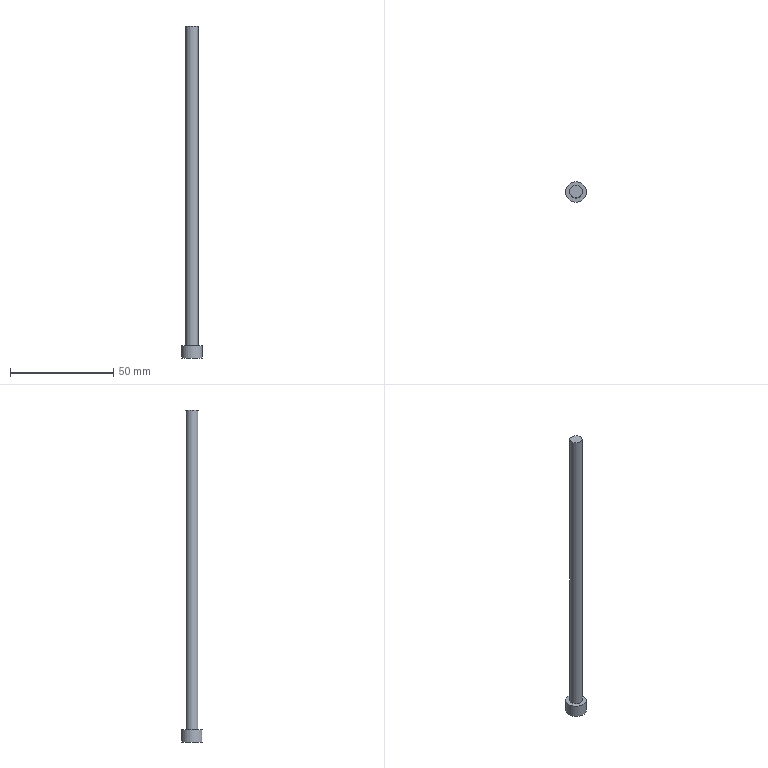Part | STEP file | DDZ6.00_id214_x_t | 1 solid | 5 faces | box 10 x 10 x 160.68 mm | volume 4845 mm3 | plane 3 | cylinder 2 | commonest cylinder face diameters 6 x1 10 x1
STEP:
#1=CARTESIAN_POINT('',(-22.,-25.,-129.5));
#2=VERTEX_POINT('',#1);
#3=CARTESIAN_POINT('',(-19.,-25.,-129.5));
#4=DIRECTION('',(0.,0.,-1.));
#5=DIRECTION('',(-1.,0.,0.));
#6=AXIS2_PLACEMENT_3D('',#3,#4,#5);
#7=CIRCLE('',#6,3.);
#8=EDGE_CURVE('',#2,#2,#7,.T.);
#9=ORIENTED_EDGE('',*,*,#8,.F.);
#10=EDGE_LOOP('',(#9));
#11=FACE_BOUND('',#10,.T.);
#12=CARTESIAN_POINT('',(-22.,-25.,25.18));
#13=VERTEX_POINT('',#12);
#14=CARTESIAN_POINT('',(-19.,-25.,25.18));
#15=DIRECTION('',(0.,0.,-1.));
#16=DIRECTION('',(-1.,0.,0.));
#17=AXIS2_PLACEMENT_3D('',#14,#15,#16);
#18=CIRCLE('',#17,3.);
#19=EDGE_CURVE('',#13,#13,#18,.T.);
#20=ORIENTED_EDGE('',*,*,#19,.T.);
#21=EDGE_LOOP('',(#20));
#22=FACE_BOUND('',#21,.T.);
#23=CARTESIAN_POINT('',(-19.,-25.,-140.5));
#24=DIRECTION('',(0.,0.,1.));
#25=DIRECTION('',(-1.,0.,0.));
#26=AXIS2_PLACEMENT_3D('',#23,#24,#25);
#27=CYLINDRICAL_SURFACE('',#26,3.);
#28=ADVANCED_FACE('',(#11,#22),#27,.T.);
#29=ORIENTED_EDGE('',*,*,#8,.T.);
#30=EDGE_LOOP('',(#29));
#31=FACE_BOUND('',#30,.T.);
#32=CARTESIAN_POINT('',(-14.,-25.,-129.5));
#33=VERTEX_POINT('',#32);
#34=CARTESIAN_POINT('',(-19.,-25.,-129.5));
#35=DIRECTION('',(0.,0.,-1.));
#36=DIRECTION('',(1.,0.,0.));
#37=AXIS2_PLACEMENT_3D('',#34,#35,#36);
#38=CIRCLE('',#37,5.);
#39=EDGE_CURVE('',#33,#33,#38,.T.);
#40=ORIENTED_EDGE('',*,*,#39,.F.);
#41=EDGE_LOOP('',(#40));
#42=FACE_BOUND('',#41,.T.);
#43=CARTESIAN_POINT('',(-19.,-25.,-129.5));
#44=DIRECTION('',(0.,0.,1.));
#45=DIRECTION('',(-1.,0.,0.));
#46=AXIS2_PLACEMENT_3D('',#43,#44,#45);
#47=PLANE('',#46);
#48=ADVANCED_FACE('',(#31,#42),#47,.T.);
#49=ORIENTED_EDGE('',*,*,#39,.T.);
#50=EDGE_LOOP('',(#49));
#51=FACE_BOUND('',#50,.T.);
#52=CARTESIAN_POINT('',(-24.,-25.,-135.5));
#53=VERTEX_POINT('',#52);
#54=CARTESIAN_POINT('',(-19.,-25.,-135.5));
#55=DIRECTION('',(0.,0.,1.));
#56=DIRECTION('',(-1.,0.,0.));
#57=AXIS2_PLACEMENT_3D('',#54,#55,#56);
#58=CIRCLE('',#57,5.);
#59=EDGE_CURVE('',#53,#53,#58,.T.);
#60=ORIENTED_EDGE('',*,*,#59,.T.);
#61=EDGE_LOOP('',(#60));
#62=FACE_BOUND('',#61,.T.);
#63=CARTESIAN_POINT('',(-19.,-25.,-135.5));
#64=DIRECTION('',(0.,0.,1.));
#65=DIRECTION('',(-1.,0.,0.));
#66=AXIS2_PLACEMENT_3D('',#63,#64,#65);
#67=CYLINDRICAL_SURFACE('',#66,5.);
#68=ADVANCED_FACE('',(#51,#62),#67,.T.);
#69=ORIENTED_EDGE('',*,*,#59,.F.);
#70=EDGE_LOOP('',(#69));
#71=FACE_OUTER_BOUND('',#70,.T.);
#72=CARTESIAN_POINT('',(-19.,-25.,-135.5));
#73=DIRECTION('',(0.,0.,-1.));
#74=DIRECTION('',(1.,0.,0.));
#75=AXIS2_PLACEMENT_3D('',#72,#73,#74);
#76=PLANE('',#75);
#77=ADVANCED_FACE('',(#71),#76,.T.);
#78=ORIENTED_EDGE('',*,*,#19,.F.);
#79=EDGE_LOOP('',(#78));
#80=FACE_OUTER_BOUND('',#79,.T.);
#81=CARTESIAN_POINT('',(-0.00001281,-37.904,25.18));
#82=DIRECTION('',(0.,0.,1.));
#83=DIRECTION('',(-1.,0.,0.));
#84=AXIS2_PLACEMENT_3D('',#81,#82,#83);
#85=PLANE('',#84);
#86=ADVANCED_FACE('',(#80),#85,.T.);
#87=CLOSED_SHELL('',(#28,#48,#68,#77,#86));
#88=MANIFOLD_SOLID_BREP('',#87);
#89=(LENGTH_UNIT()NAMED_UNIT(*)SI_UNIT(.MILLI.,.METRE.));
#90=UNCERTAINTY_MEASURE_WITH_UNIT(LENGTH_MEASURE(0.00002),#89,'','');
#91=(NAMED_UNIT(*)PLANE_ANGLE_UNIT()SI_UNIT($,.RADIAN.));
#92=PLANE_ANGLE_MEASURE_WITH_UNIT(PLANE_ANGLE_MEASURE(0.01745),#91);
#93=DIMENSIONAL_EXPONENTS(0.,0.,0.,0.,0.,0.,0.);
#94=(CONVERSION_BASED_UNIT('DEGREE',#92)NAMED_UNIT(#93)PLANE_ANGLE_UNIT());
#95=(NAMED_UNIT(*)SI_UNIT($,.STERADIAN.)SOLID_ANGLE_UNIT());
#96=(GEOMETRIC_REPRESENTATION_CONTEXT(3)GLOBAL_UNCERTAINTY_ASSIGNED_CONTEXT((#90))GLOBAL_UNIT_ASSIGNED_CONTEXT((#89,#94,#95))REPRESENTATION_CONTEXT('',''));
#97=ADVANCED_BREP_SHAPE_REPRESENTATION('',(#88),#96);